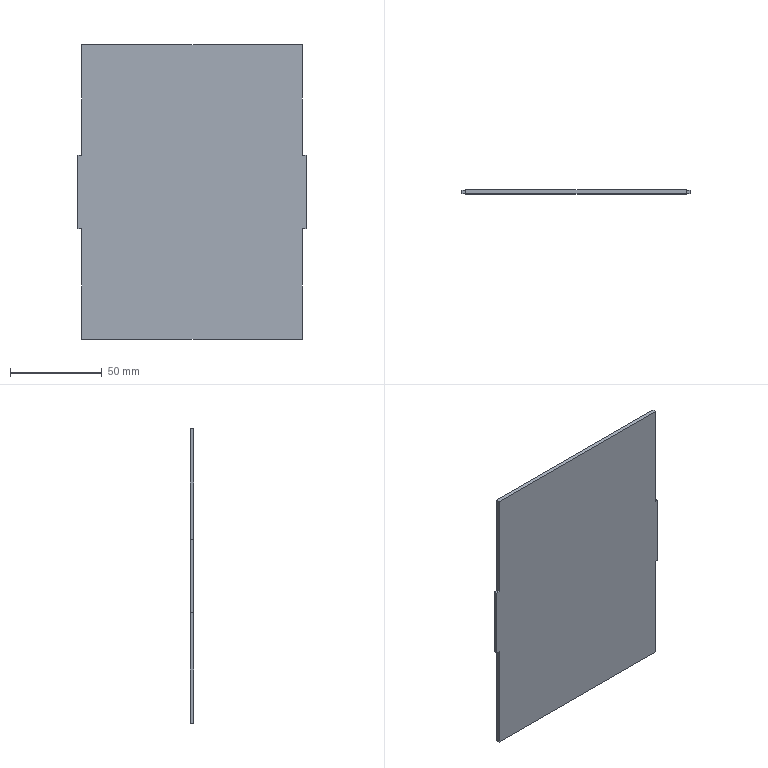Part | STEP file | JBJ-P-1003-03 | 1 solid | 14 faces | box 124 x 2 x 160 mm | volume 38720 mm3 | plane 14
STEP:
#1=CARTESIAN_POINT('',(60.,0.,80.));
#2=VERTEX_POINT('',#1);
#3=CARTESIAN_POINT('',(60.,0.,20.));
#4=VERTEX_POINT('',#3);
#5=CARTESIAN_POINT('',(60.,0.,-80.));
#6=DIRECTION('',(0.,0.,-1.));
#7=VECTOR('',#6,1000.);
#8=LINE('',#5,#7);
#9=EDGE_CURVE('',#2,#4,#8,.T.);
#10=ORIENTED_EDGE('',*,*,#9,.T.);
#11=CARTESIAN_POINT('',(60.,2.,20.));
#12=VERTEX_POINT('',#11);
#13=CARTESIAN_POINT('',(60.,2.,20.));
#14=DIRECTION('',(0.,1.,0.));
#15=VECTOR('',#14,1000.);
#16=LINE('',#13,#15);
#17=EDGE_CURVE('',#4,#12,#16,.T.);
#18=ORIENTED_EDGE('',*,*,#17,.T.);
#19=CARTESIAN_POINT('',(60.,2.,80.));
#20=VERTEX_POINT('',#19);
#21=CARTESIAN_POINT('',(60.,2.,-80.));
#22=DIRECTION('',(0.,0.,-1.));
#23=VECTOR('',#22,1000.);
#24=LINE('',#21,#23);
#25=EDGE_CURVE('',#20,#12,#24,.T.);
#26=ORIENTED_EDGE('',*,*,#25,.F.);
#27=CARTESIAN_POINT('',(60.,2.,80.));
#28=DIRECTION('',(0.,-1.,0.));
#29=VECTOR('',#28,1000.);
#30=LINE('',#27,#29);
#31=EDGE_CURVE('',#20,#2,#30,.T.);
#32=ORIENTED_EDGE('',*,*,#31,.T.);
#33=EDGE_LOOP('',(#10,#18,#26,#32));
#34=FACE_OUTER_BOUND('',#33,.T.);
#35=CARTESIAN_POINT('',(60.,2.,-80.));
#36=DIRECTION('',(-1.,0.,0.));
#37=DIRECTION('',(0.,0.,1.));
#38=AXIS2_PLACEMENT_3D('',#35,#36,#37);
#39=PLANE('',#38);
#40=ADVANCED_FACE('',(#34),#39,.F.);
#41=CARTESIAN_POINT('',(-60.,0.,20.));
#42=VERTEX_POINT('',#41);
#43=CARTESIAN_POINT('',(-60.,2.,20.));
#44=VERTEX_POINT('',#43);
#45=CARTESIAN_POINT('',(-60.,2.,20.));
#46=DIRECTION('',(0.,1.,0.));
#47=VECTOR('',#46,1000.);
#48=LINE('',#45,#47);
#49=EDGE_CURVE('',#42,#44,#48,.T.);
#50=ORIENTED_EDGE('',*,*,#49,.F.);
#51=CARTESIAN_POINT('',(-60.,0.,80.));
#52=VERTEX_POINT('',#51);
#53=CARTESIAN_POINT('',(-60.,0.,-80.));
#54=DIRECTION('',(0.,0.,1.));
#55=VECTOR('',#54,1000.);
#56=LINE('',#53,#55);
#57=EDGE_CURVE('',#42,#52,#56,.T.);
#58=ORIENTED_EDGE('',*,*,#57,.T.);
#59=CARTESIAN_POINT('',(-60.,2.,80.));
#60=VERTEX_POINT('',#59);
#61=CARTESIAN_POINT('',(-60.,2.,80.));
#62=DIRECTION('',(0.,-1.,0.));
#63=VECTOR('',#62,1000.);
#64=LINE('',#61,#63);
#65=EDGE_CURVE('',#60,#52,#64,.T.);
#66=ORIENTED_EDGE('',*,*,#65,.F.);
#67=CARTESIAN_POINT('',(-60.,2.,-80.));
#68=DIRECTION('',(0.,0.,1.));
#69=VECTOR('',#68,1000.);
#70=LINE('',#67,#69);
#71=EDGE_CURVE('',#44,#60,#70,.T.);
#72=ORIENTED_EDGE('',*,*,#71,.F.);
#73=EDGE_LOOP('',(#50,#58,#66,#72));
#74=FACE_OUTER_BOUND('',#73,.T.);
#75=CARTESIAN_POINT('',(-60.,2.,-80.));
#76=DIRECTION('',(1.,0.,0.));
#77=DIRECTION('',(0.,0.,-1.));
#78=AXIS2_PLACEMENT_3D('',#75,#76,#77);
#79=PLANE('',#78);
#80=ADVANCED_FACE('',(#74),#79,.F.);
#81=CARTESIAN_POINT('',(-60.,2.,-20.));
#82=VERTEX_POINT('',#81);
#83=CARTESIAN_POINT('',(-60.,0.,-20.));
#84=VERTEX_POINT('',#83);
#85=CARTESIAN_POINT('',(-60.,2.,-20.));
#86=DIRECTION('',(0.,-1.,0.));
#87=VECTOR('',#86,1000.);
#88=LINE('',#85,#87);
#89=EDGE_CURVE('',#82,#84,#88,.T.);
#90=ORIENTED_EDGE('',*,*,#89,.F.);
#91=CARTESIAN_POINT('',(-60.,2.,-80.));
#92=VERTEX_POINT('',#91);
#93=CARTESIAN_POINT('',(-60.,2.,-80.));
#94=DIRECTION('',(0.,0.,1.));
#95=VECTOR('',#94,1000.);
#96=LINE('',#93,#95);
#97=EDGE_CURVE('',#92,#82,#96,.T.);
#98=ORIENTED_EDGE('',*,*,#97,.F.);
#99=CARTESIAN_POINT('',(-60.,0.,-80.));
#100=VERTEX_POINT('',#99);
#101=CARTESIAN_POINT('',(-60.,2.,-80.));
#102=DIRECTION('',(0.,-1.,0.));
#103=VECTOR('',#102,1000.);
#104=LINE('',#101,#103);
#105=EDGE_CURVE('',#92,#100,#104,.T.);
#106=ORIENTED_EDGE('',*,*,#105,.T.);
#107=CARTESIAN_POINT('',(-60.,0.,-80.));
#108=DIRECTION('',(0.,0.,1.));
#109=VECTOR('',#108,1000.);
#110=LINE('',#107,#109);
#111=EDGE_CURVE('',#100,#84,#110,.T.);
#112=ORIENTED_EDGE('',*,*,#111,.T.);
#113=EDGE_LOOP('',(#90,#98,#106,#112));
#114=FACE_OUTER_BOUND('',#113,.T.);
#115=CARTESIAN_POINT('',(-60.,2.,-80.));
#116=DIRECTION('',(1.,0.,0.));
#117=DIRECTION('',(0.,0.,-1.));
#118=AXIS2_PLACEMENT_3D('',#115,#116,#117);
#119=PLANE('',#118);
#120=ADVANCED_FACE('',(#114),#119,.F.);
#121=CARTESIAN_POINT('',(60.,2.,-20.));
#122=VERTEX_POINT('',#121);
#123=CARTESIAN_POINT('',(60.,2.,-80.));
#124=VERTEX_POINT('',#123);
#125=CARTESIAN_POINT('',(60.,2.,-80.));
#126=DIRECTION('',(0.,0.,-1.));
#127=VECTOR('',#126,1000.);
#128=LINE('',#125,#127);
#129=EDGE_CURVE('',#122,#124,#128,.T.);
#130=ORIENTED_EDGE('',*,*,#129,.F.);
#131=CARTESIAN_POINT('',(60.,0.,-20.));
#132=VERTEX_POINT('',#131);
#133=CARTESIAN_POINT('',(60.,2.,-20.));
#134=DIRECTION('',(0.,-1.,0.));
#135=VECTOR('',#134,1000.);
#136=LINE('',#133,#135);
#137=EDGE_CURVE('',#122,#132,#136,.T.);
#138=ORIENTED_EDGE('',*,*,#137,.T.);
#139=CARTESIAN_POINT('',(60.,0.,-80.));
#140=VERTEX_POINT('',#139);
#141=CARTESIAN_POINT('',(60.,0.,-80.));
#142=DIRECTION('',(0.,0.,-1.));
#143=VECTOR('',#142,1000.);
#144=LINE('',#141,#143);
#145=EDGE_CURVE('',#132,#140,#144,.T.);
#146=ORIENTED_EDGE('',*,*,#145,.T.);
#147=CARTESIAN_POINT('',(60.,2.,-80.));
#148=DIRECTION('',(0.,-1.,0.));
#149=VECTOR('',#148,1000.);
#150=LINE('',#147,#149);
#151=EDGE_CURVE('',#124,#140,#150,.T.);
#152=ORIENTED_EDGE('',*,*,#151,.F.);
#153=EDGE_LOOP('',(#130,#138,#146,#152));
#154=FACE_OUTER_BOUND('',#153,.T.);
#155=CARTESIAN_POINT('',(60.,2.,-80.));
#156=DIRECTION('',(-1.,0.,0.));
#157=DIRECTION('',(0.,0.,1.));
#158=AXIS2_PLACEMENT_3D('',#155,#156,#157);
#159=PLANE('',#158);
#160=ADVANCED_FACE('',(#154),#159,.F.);
#161=CARTESIAN_POINT('',(-60.,0.,-80.));
#162=DIRECTION('',(-1.,0.,0.));
#163=VECTOR('',#162,1000.);
#164=LINE('',#161,#163);
#165=EDGE_CURVE('',#140,#100,#164,.T.);
#166=ORIENTED_EDGE('',*,*,#165,.T.);
#167=ORIENTED_EDGE('',*,*,#105,.F.);
#168=CARTESIAN_POINT('',(-60.,2.,-80.));
#169=DIRECTION('',(-1.,0.,0.));
#170=VECTOR('',#169,1000.);
#171=LINE('',#168,#170);
#172=EDGE_CURVE('',#124,#92,#171,.T.);
#173=ORIENTED_EDGE('',*,*,#172,.F.);
#174=ORIENTED_EDGE('',*,*,#151,.T.);
#175=EDGE_LOOP('',(#166,#167,#173,#174));
#176=FACE_OUTER_BOUND('',#175,.T.);
#177=CARTESIAN_POINT('',(-60.,2.,-80.));
#178=DIRECTION('',(0.,0.,1.));
#179=DIRECTION('',(1.,0.,0.));
#180=AXIS2_PLACEMENT_3D('',#177,#178,#179);
#181=PLANE('',#180);
#182=ADVANCED_FACE('',(#176),#181,.F.);
#183=CARTESIAN_POINT('',(-60.,0.,80.));
#184=DIRECTION('',(1.,0.,0.));
#185=VECTOR('',#184,1000.);
#186=LINE('',#183,#185);
#187=EDGE_CURVE('',#52,#2,#186,.T.);
#188=ORIENTED_EDGE('',*,*,#187,.T.);
#189=ORIENTED_EDGE('',*,*,#31,.F.);
#190=CARTESIAN_POINT('',(-60.,2.,80.));
#191=DIRECTION('',(1.,0.,0.));
#192=VECTOR('',#191,1000.);
#193=LINE('',#190,#192);
#194=EDGE_CURVE('',#60,#20,#193,.T.);
#195=ORIENTED_EDGE('',*,*,#194,.F.);
#196=ORIENTED_EDGE('',*,*,#65,.T.);
#197=EDGE_LOOP('',(#188,#189,#195,#196));
#198=FACE_OUTER_BOUND('',#197,.T.);
#199=CARTESIAN_POINT('',(-60.,2.,80.));
#200=DIRECTION('',(0.,0.,-1.));
#201=DIRECTION('',(-1.,0.,0.));
#202=AXIS2_PLACEMENT_3D('',#199,#200,#201);
#203=PLANE('',#202);
#204=ADVANCED_FACE('',(#198),#203,.F.);
#205=ORIENTED_EDGE('',*,*,#25,.T.);
#206=CARTESIAN_POINT('',(62.,2.,20.));
#207=VERTEX_POINT('',#206);
#208=CARTESIAN_POINT('',(62.,2.,20.));
#209=DIRECTION('',(-1.,0.,0.));
#210=VECTOR('',#209,1000.);
#211=LINE('',#208,#210);
#212=EDGE_CURVE('',#207,#12,#211,.T.);
#213=ORIENTED_EDGE('',*,*,#212,.F.);
#214=CARTESIAN_POINT('',(62.,2.,-20.));
#215=VERTEX_POINT('',#214);
#216=CARTESIAN_POINT('',(62.,2.,20.));
#217=DIRECTION('',(0.,0.,-1.));
#218=VECTOR('',#217,1000.);
#219=LINE('',#216,#218);
#220=EDGE_CURVE('',#207,#215,#219,.T.);
#221=ORIENTED_EDGE('',*,*,#220,.T.);
#222=CARTESIAN_POINT('',(62.,2.,-20.));
#223=DIRECTION('',(-1.,0.,0.));
#224=VECTOR('',#223,1000.);
#225=LINE('',#222,#224);
#226=EDGE_CURVE('',#215,#122,#225,.T.);
#227=ORIENTED_EDGE('',*,*,#226,.T.);
#228=ORIENTED_EDGE('',*,*,#129,.T.);
#229=ORIENTED_EDGE('',*,*,#172,.T.);
#230=ORIENTED_EDGE('',*,*,#97,.T.);
#231=CARTESIAN_POINT('',(-62.,2.,-20.));
#232=VERTEX_POINT('',#231);
#233=CARTESIAN_POINT('',(-62.,2.,-20.));
#234=DIRECTION('',(1.,0.,0.));
#235=VECTOR('',#234,1000.);
#236=LINE('',#233,#235);
#237=EDGE_CURVE('',#232,#82,#236,.T.);
#238=ORIENTED_EDGE('',*,*,#237,.F.);
#239=CARTESIAN_POINT('',(-62.,2.,20.));
#240=VERTEX_POINT('',#239);
#241=CARTESIAN_POINT('',(-62.,2.,20.));
#242=DIRECTION('',(0.,0.,-1.));
#243=VECTOR('',#242,1000.);
#244=LINE('',#241,#243);
#245=EDGE_CURVE('',#240,#232,#244,.T.);
#246=ORIENTED_EDGE('',*,*,#245,.F.);
#247=CARTESIAN_POINT('',(-62.,2.,20.));
#248=DIRECTION('',(1.,0.,0.));
#249=VECTOR('',#248,1000.);
#250=LINE('',#247,#249);
#251=EDGE_CURVE('',#240,#44,#250,.T.);
#252=ORIENTED_EDGE('',*,*,#251,.T.);
#253=ORIENTED_EDGE('',*,*,#71,.T.);
#254=ORIENTED_EDGE('',*,*,#194,.T.);
#255=EDGE_LOOP('',(#205,#213,#221,#227,#228,#229,#230,#238,#246,#252,#253,#254));
#256=FACE_OUTER_BOUND('',#255,.T.);
#257=CARTESIAN_POINT('',(0.,2.,0.));
#258=DIRECTION('',(0.,1.,0.));
#259=DIRECTION('',(0.,0.,1.));
#260=AXIS2_PLACEMENT_3D('',#257,#258,#259);
#261=PLANE('',#260);
#262=ADVANCED_FACE('',(#256),#261,.T.);
#263=ORIENTED_EDGE('',*,*,#9,.F.);
#264=ORIENTED_EDGE('',*,*,#187,.F.);
#265=ORIENTED_EDGE('',*,*,#57,.F.);
#266=CARTESIAN_POINT('',(-62.,0.,20.));
#267=VERTEX_POINT('',#266);
#268=CARTESIAN_POINT('',(-62.,0.,20.));
#269=DIRECTION('',(1.,0.,0.));
#270=VECTOR('',#269,1000.);
#271=LINE('',#268,#270);
#272=EDGE_CURVE('',#267,#42,#271,.T.);
#273=ORIENTED_EDGE('',*,*,#272,.F.);
#274=CARTESIAN_POINT('',(-62.,0.,-20.));
#275=VERTEX_POINT('',#274);
#276=CARTESIAN_POINT('',(-62.,0.,20.));
#277=DIRECTION('',(0.,0.,1.));
#278=VECTOR('',#277,1000.);
#279=LINE('',#276,#278);
#280=EDGE_CURVE('',#275,#267,#279,.T.);
#281=ORIENTED_EDGE('',*,*,#280,.F.);
#282=CARTESIAN_POINT('',(-62.,0.,-20.));
#283=DIRECTION('',(1.,0.,0.));
#284=VECTOR('',#283,1000.);
#285=LINE('',#282,#284);
#286=EDGE_CURVE('',#275,#84,#285,.T.);
#287=ORIENTED_EDGE('',*,*,#286,.T.);
#288=ORIENTED_EDGE('',*,*,#111,.F.);
#289=ORIENTED_EDGE('',*,*,#165,.F.);
#290=ORIENTED_EDGE('',*,*,#145,.F.);
#291=CARTESIAN_POINT('',(62.,0.,-20.));
#292=VERTEX_POINT('',#291);
#293=CARTESIAN_POINT('',(62.,0.,-20.));
#294=DIRECTION('',(-1.,0.,0.));
#295=VECTOR('',#294,1000.);
#296=LINE('',#293,#295);
#297=EDGE_CURVE('',#292,#132,#296,.T.);
#298=ORIENTED_EDGE('',*,*,#297,.F.);
#299=CARTESIAN_POINT('',(62.,0.,20.));
#300=VERTEX_POINT('',#299);
#301=CARTESIAN_POINT('',(62.,0.,20.));
#302=DIRECTION('',(0.,0.,1.));
#303=VECTOR('',#302,1000.);
#304=LINE('',#301,#303);
#305=EDGE_CURVE('',#292,#300,#304,.T.);
#306=ORIENTED_EDGE('',*,*,#305,.T.);
#307=CARTESIAN_POINT('',(62.,0.,20.));
#308=DIRECTION('',(-1.,0.,0.));
#309=VECTOR('',#308,1000.);
#310=LINE('',#307,#309);
#311=EDGE_CURVE('',#300,#4,#310,.T.);
#312=ORIENTED_EDGE('',*,*,#311,.T.);
#313=EDGE_LOOP('',(#263,#264,#265,#273,#281,#287,#288,#289,#290,#298,#306,#312));
#314=FACE_OUTER_BOUND('',#313,.T.);
#315=CARTESIAN_POINT('',(0.,0.,0.));
#316=DIRECTION('',(0.,1.,0.));
#317=DIRECTION('',(0.,0.,1.));
#318=AXIS2_PLACEMENT_3D('',#315,#316,#317);
#319=PLANE('',#318);
#320=ADVANCED_FACE('',(#314),#319,.F.);
#321=ORIENTED_EDGE('',*,*,#49,.T.);
#322=ORIENTED_EDGE('',*,*,#251,.F.);
#323=CARTESIAN_POINT('',(-62.,2.,20.));
#324=DIRECTION('',(0.,1.,0.));
#325=VECTOR('',#324,1000.);
#326=LINE('',#323,#325);
#327=EDGE_CURVE('',#267,#240,#326,.T.);
#328=ORIENTED_EDGE('',*,*,#327,.F.);
#329=ORIENTED_EDGE('',*,*,#272,.T.);
#330=EDGE_LOOP('',(#321,#322,#328,#329));
#331=FACE_OUTER_BOUND('',#330,.T.);
#332=CARTESIAN_POINT('',(-62.,2.,20.));
#333=DIRECTION('',(0.,0.,-1.));
#334=DIRECTION('',(0.,1.,0.));
#335=AXIS2_PLACEMENT_3D('',#332,#333,#334);
#336=PLANE('',#335);
#337=ADVANCED_FACE('',(#331),#336,.F.);
#338=ORIENTED_EDGE('',*,*,#89,.T.);
#339=ORIENTED_EDGE('',*,*,#286,.F.);
#340=CARTESIAN_POINT('',(-62.,2.,-20.));
#341=DIRECTION('',(0.,-1.,0.));
#342=VECTOR('',#341,1000.);
#343=LINE('',#340,#342);
#344=EDGE_CURVE('',#232,#275,#343,.T.);
#345=ORIENTED_EDGE('',*,*,#344,.F.);
#346=ORIENTED_EDGE('',*,*,#237,.T.);
#347=EDGE_LOOP('',(#338,#339,#345,#346));
#348=FACE_OUTER_BOUND('',#347,.T.);
#349=CARTESIAN_POINT('',(-62.,2.,-20.));
#350=DIRECTION('',(0.,0.,1.));
#351=DIRECTION('',(1.,0.,0.));
#352=AXIS2_PLACEMENT_3D('',#349,#350,#351);
#353=PLANE('',#352);
#354=ADVANCED_FACE('',(#348),#353,.F.);
#355=ORIENTED_EDGE('',*,*,#327,.T.);
#356=ORIENTED_EDGE('',*,*,#245,.T.);
#357=ORIENTED_EDGE('',*,*,#344,.T.);
#358=ORIENTED_EDGE('',*,*,#280,.T.);
#359=EDGE_LOOP('',(#355,#356,#357,#358));
#360=FACE_OUTER_BOUND('',#359,.T.);
#361=CARTESIAN_POINT('',(-62.,0.,0.));
#362=DIRECTION('',(1.,0.,0.));
#363=DIRECTION('',(0.,0.,-1.));
#364=AXIS2_PLACEMENT_3D('',#361,#362,#363);
#365=PLANE('',#364);
#366=ADVANCED_FACE('',(#360),#365,.F.);
#367=ORIENTED_EDGE('',*,*,#17,.F.);
#368=ORIENTED_EDGE('',*,*,#311,.F.);
#369=CARTESIAN_POINT('',(62.,2.,20.));
#370=DIRECTION('',(0.,1.,0.));
#371=VECTOR('',#370,1000.);
#372=LINE('',#369,#371);
#373=EDGE_CURVE('',#300,#207,#372,.T.);
#374=ORIENTED_EDGE('',*,*,#373,.T.);
#375=ORIENTED_EDGE('',*,*,#212,.T.);
#376=EDGE_LOOP('',(#367,#368,#374,#375));
#377=FACE_OUTER_BOUND('',#376,.T.);
#378=CARTESIAN_POINT('',(62.,2.,20.));
#379=DIRECTION('',(0.,0.,1.));
#380=DIRECTION('',(0.,-1.,0.));
#381=AXIS2_PLACEMENT_3D('',#378,#379,#380);
#382=PLANE('',#381);
#383=ADVANCED_FACE('',(#377),#382,.T.);
#384=ORIENTED_EDGE('',*,*,#137,.F.);
#385=ORIENTED_EDGE('',*,*,#226,.F.);
#386=CARTESIAN_POINT('',(62.,2.,-20.));
#387=DIRECTION('',(0.,-1.,0.));
#388=VECTOR('',#387,1000.);
#389=LINE('',#386,#388);
#390=EDGE_CURVE('',#215,#292,#389,.T.);
#391=ORIENTED_EDGE('',*,*,#390,.T.);
#392=ORIENTED_EDGE('',*,*,#297,.T.);
#393=EDGE_LOOP('',(#384,#385,#391,#392));
#394=FACE_OUTER_BOUND('',#393,.T.);
#395=CARTESIAN_POINT('',(62.,2.,-20.));
#396=DIRECTION('',(0.,0.,-1.));
#397=DIRECTION('',(-1.,0.,0.));
#398=AXIS2_PLACEMENT_3D('',#395,#396,#397);
#399=PLANE('',#398);
#400=ADVANCED_FACE('',(#394),#399,.T.);
#401=ORIENTED_EDGE('',*,*,#373,.F.);
#402=ORIENTED_EDGE('',*,*,#305,.F.);
#403=ORIENTED_EDGE('',*,*,#390,.F.);
#404=ORIENTED_EDGE('',*,*,#220,.F.);
#405=EDGE_LOOP('',(#401,#402,#403,#404));
#406=FACE_OUTER_BOUND('',#405,.T.);
#407=CARTESIAN_POINT('',(62.,0.,0.));
#408=DIRECTION('',(-1.,0.,0.));
#409=DIRECTION('',(0.,0.,-1.));
#410=AXIS2_PLACEMENT_3D('',#407,#408,#409);
#411=PLANE('',#410);
#412=ADVANCED_FACE('',(#406),#411,.F.);
#413=CLOSED_SHELL('',(#40,#80,#120,#160,#182,#204,#262,#320,#337,#354,#366,#383,#400,#412));
#414=MANIFOLD_SOLID_BREP('',#413);
#415=CARTESIAN_POINT('',(0.,0.,0.));
#416=DIRECTION('',(0.,0.,1.));
#417=DIRECTION('',(1.,0.,0.));
#418=AXIS2_PLACEMENT_3D('',#415,#416,#417);
#419=(LENGTH_UNIT()NAMED_UNIT(*)SI_UNIT(.MILLI.,.METRE.));
#420=UNCERTAINTY_MEASURE_WITH_UNIT(LENGTH_MEASURE(0.00001),#419,'','');
#421=(NAMED_UNIT(*)PLANE_ANGLE_UNIT()SI_UNIT($,.RADIAN.));
#422=(NAMED_UNIT(*)SI_UNIT($,.STERADIAN.)SOLID_ANGLE_UNIT());
#423=(GEOMETRIC_REPRESENTATION_CONTEXT(3)GLOBAL_UNCERTAINTY_ASSIGNED_CONTEXT((#420))GLOBAL_UNIT_ASSIGNED_CONTEXT((#419,#421,#422))REPRESENTATION_CONTEXT('',''));
#424=ADVANCED_BREP_SHAPE_REPRESENTATION('',(#414,#418),#423);